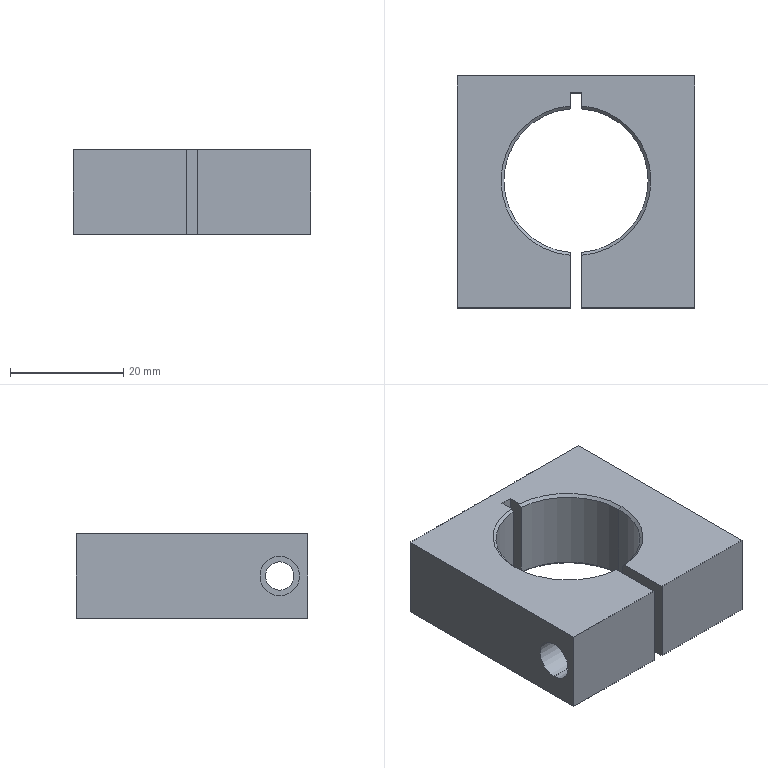Part | SolidWorks | features HoleWzd 3, Chamfer 2, ICE 2, Extrusion 1 | 1 solid | 33 faces | box 42 x 41 x 15 mm | volume 15925 mm3 | plane 12 | cylinder 11 | cone 10 | commonest cylinder face diameters 5 x6 25.5 x3 7 x2
STEP:
#1=CARTESIAN_POINT('',(8.25,22.5,0.5));
#2=VERTEX_POINT('',#1);
#3=CARTESIAN_POINT('',(20.,35.211,0.5));
#4=VERTEX_POINT('',#3);
#5=CARTESIAN_POINT('',(21.,22.5,0.5));
#6=DIRECTION('',(0.,0.,-1.));
#7=DIRECTION('',(-1.,0.,0.));
#8=AXIS2_PLACEMENT_3D('',#5,#6,#7);
#9=CIRCLE('',#8,12.75);
#10=EDGE_CURVE('',#2,#4,#9,.T.);
#11=ORIENTED_EDGE('',*,*,#10,.F.);
#12=CARTESIAN_POINT('',(7.75,22.5,0.));
#13=VERTEX_POINT('',#12);
#14=CARTESIAN_POINT('',(7.75,22.5,0.));
#15=DIRECTION('',(-0.7071,0.,-0.7071));
#16=VECTOR('',#15,1000.);
#17=LINE('',#14,#16);
#18=EDGE_CURVE('',#2,#13,#17,.T.);
#19=ORIENTED_EDGE('',*,*,#18,.T.);
#20=CARTESIAN_POINT('',(20.,35.712,0.));
#21=VERTEX_POINT('',#20);
#22=CARTESIAN_POINT('',(21.,22.5,0.));
#23=DIRECTION('',(0.,0.,1.));
#24=DIRECTION('',(-1.,0.,0.));
#25=AXIS2_PLACEMENT_3D('',#22,#23,#24);
#26=CIRCLE('',#25,13.25);
#27=EDGE_CURVE('',#21,#13,#26,.T.);
#28=ORIENTED_EDGE('',*,*,#27,.F.);
#29=CARTESIAN_POINT('',(20.,35.211,0.5));
#30=CARTESIAN_POINT('',(20.,35.378,0.3333));
#31=CARTESIAN_POINT('',(20.,35.545,0.1667));
#32=CARTESIAN_POINT('',(20.,35.712,0.));
#33=B_SPLINE_CURVE_WITH_KNOTS('',3,(#29,#30,#31,#32),.UNSPECIFIED.,.F.,.F.,(4,4),(0.,0.0007082),.UNSPECIFIED.);
#34=EDGE_CURVE('',#4,#21,#33,.T.);
#35=ORIENTED_EDGE('',*,*,#34,.F.);
#36=EDGE_LOOP('',(#11,#19,#28,#35));
#37=FACE_OUTER_BOUND('',#36,.T.);
#38=CARTESIAN_POINT('',(21.,22.5,0.));
#39=DIRECTION('',(0.,0.,-1.));
#40=DIRECTION('',(-1.,0.,0.));
#41=AXIS2_PLACEMENT_3D('',#38,#39,#40);
#42=CONICAL_SURFACE('',#41,13.25,0.7854);
#43=ADVANCED_FACE('',(#37),#42,.F.);
#44=CARTESIAN_POINT('',(33.75,22.5,14.5));
#45=VERTEX_POINT('',#44);
#46=CARTESIAN_POINT('',(22.,35.211,14.5));
#47=VERTEX_POINT('',#46);
#48=CARTESIAN_POINT('',(21.,22.5,14.5));
#49=DIRECTION('',(0.,0.,1.));
#50=DIRECTION('',(-1.,0.,0.));
#51=AXIS2_PLACEMENT_3D('',#48,#49,#50);
#52=CIRCLE('',#51,12.75);
#53=EDGE_CURVE('',#45,#47,#52,.T.);
#54=ORIENTED_EDGE('',*,*,#53,.F.);
#55=CARTESIAN_POINT('',(34.25,22.5,15.));
#56=VERTEX_POINT('',#55);
#57=CARTESIAN_POINT('',(33.75,22.5,14.5));
#58=DIRECTION('',(0.7071,0.,0.7071));
#59=VECTOR('',#58,1000.);
#60=LINE('',#57,#59);
#61=EDGE_CURVE('',#45,#56,#60,.T.);
#62=ORIENTED_EDGE('',*,*,#61,.T.);
#63=CARTESIAN_POINT('',(22.,35.712,15.));
#64=VERTEX_POINT('',#63);
#65=CARTESIAN_POINT('',(21.,22.5,15.));
#66=DIRECTION('',(0.,0.,-1.));
#67=DIRECTION('',(-1.,0.,0.));
#68=AXIS2_PLACEMENT_3D('',#65,#66,#67);
#69=CIRCLE('',#68,13.25);
#70=EDGE_CURVE('',#64,#56,#69,.T.);
#71=ORIENTED_EDGE('',*,*,#70,.F.);
#72=CARTESIAN_POINT('',(22.,35.211,14.5));
#73=CARTESIAN_POINT('',(22.,35.378,14.667));
#74=CARTESIAN_POINT('',(22.,35.545,14.833));
#75=CARTESIAN_POINT('',(22.,35.712,15.));
#76=B_SPLINE_CURVE_WITH_KNOTS('',3,(#72,#73,#74,#75),.UNSPECIFIED.,.F.,.F.,(4,4),(0.,0.0007082),.UNSPECIFIED.);
#77=EDGE_CURVE('',#47,#64,#76,.T.);
#78=ORIENTED_EDGE('',*,*,#77,.F.);
#79=EDGE_LOOP('',(#54,#62,#71,#78));
#80=FACE_OUTER_BOUND('',#79,.T.);
#81=CARTESIAN_POINT('',(21.,22.5,14.5));
#82=DIRECTION('',(0.,0.,1.));
#83=DIRECTION('',(1.,0.,0.));
#84=AXIS2_PLACEMENT_3D('',#81,#82,#83);
#85=CONICAL_SURFACE('',#84,12.75,0.7854);
#86=ADVANCED_FACE('',(#80),#85,.F.);
#87=CARTESIAN_POINT('',(42.,5.,5.));
#88=VERTEX_POINT('',#87);
#89=CARTESIAN_POINT('',(42.,5.,10.));
#90=VERTEX_POINT('',#89);
#91=CARTESIAN_POINT('',(42.,5.,7.5));
#92=DIRECTION('',(-1.,0.,0.));
#93=DIRECTION('',(0.,0.,1.));
#94=AXIS2_PLACEMENT_3D('',#91,#92,#93);
#95=CIRCLE('',#94,2.5);
#96=EDGE_CURVE('',#88,#90,#95,.T.);
#97=ORIENTED_EDGE('',*,*,#96,.F.);
#98=CARTESIAN_POINT('',(22.,5.,5.));
#99=VERTEX_POINT('',#98);
#100=CARTESIAN_POINT('',(22.,5.,5.));
#101=DIRECTION('',(-1.,0.,0.));
#102=VECTOR('',#101,1000.);
#103=LINE('',#100,#102);
#104=EDGE_CURVE('',#88,#99,#103,.T.);
#105=ORIENTED_EDGE('',*,*,#104,.T.);
#106=CARTESIAN_POINT('',(22.,5.,10.));
#107=VERTEX_POINT('',#106);
#108=CARTESIAN_POINT('',(22.,5.,7.5));
#109=DIRECTION('',(-1.,0.,0.));
#110=DIRECTION('',(0.,0.,1.));
#111=AXIS2_PLACEMENT_3D('',#108,#109,#110);
#112=CIRCLE('',#111,2.5);
#113=EDGE_CURVE('',#99,#107,#112,.T.);
#114=ORIENTED_EDGE('',*,*,#113,.T.);
#115=CARTESIAN_POINT('',(22.,5.,10.));
#116=DIRECTION('',(-1.,0.,0.));
#117=VECTOR('',#116,1000.);
#118=LINE('',#115,#117);
#119=EDGE_CURVE('',#90,#107,#118,.T.);
#120=ORIENTED_EDGE('',*,*,#119,.F.);
#121=EDGE_LOOP('',(#97,#105,#114,#120));
#122=FACE_OUTER_BOUND('',#121,.T.);
#123=CARTESIAN_POINT('',(22.,5.,7.5));
#124=DIRECTION('',(-1.,0.,0.));
#125=DIRECTION('',(0.,0.,1.));
#126=AXIS2_PLACEMENT_3D('',#123,#124,#125);
#127=CYLINDRICAL_SURFACE('',#126,2.5);
#128=ADVANCED_FACE('',(#122),#127,.F.);
#129=CARTESIAN_POINT('',(20.,5.,4.));
#130=VERTEX_POINT('',#129);
#131=CARTESIAN_POINT('',(20.,5.,11.));
#132=VERTEX_POINT('',#131);
#133=CARTESIAN_POINT('',(20.,5.,7.5));
#134=DIRECTION('',(-1.,0.,0.));
#135=DIRECTION('',(0.,-1.,0.));
#136=AXIS2_PLACEMENT_3D('',#133,#134,#135);
#137=CIRCLE('',#136,3.5);
#138=EDGE_CURVE('',#130,#132,#137,.T.);
#139=ORIENTED_EDGE('',*,*,#138,.F.);
#140=CARTESIAN_POINT('',(0.,5.,4.));
#141=VERTEX_POINT('',#140);
#142=CARTESIAN_POINT('',(0.,5.,4.));
#143=DIRECTION('',(-1.,0.,0.));
#144=VECTOR('',#143,1000.);
#145=LINE('',#142,#144);
#146=EDGE_CURVE('',#130,#141,#145,.T.);
#147=ORIENTED_EDGE('',*,*,#146,.T.);
#148=CARTESIAN_POINT('',(0.,5.,11.));
#149=VERTEX_POINT('',#148);
#150=CARTESIAN_POINT('',(0.,5.,7.5));
#151=DIRECTION('',(-1.,0.,0.));
#152=DIRECTION('',(0.,0.,1.));
#153=AXIS2_PLACEMENT_3D('',#150,#151,#152);
#154=CIRCLE('',#153,3.5);
#155=EDGE_CURVE('',#141,#149,#154,.T.);
#156=ORIENTED_EDGE('',*,*,#155,.T.);
#157=CARTESIAN_POINT('',(0.,5.,11.));
#158=DIRECTION('',(-1.,0.,0.));
#159=VECTOR('',#158,1000.);
#160=LINE('',#157,#159);
#161=EDGE_CURVE('',#132,#149,#160,.T.);
#162=ORIENTED_EDGE('',*,*,#161,.F.);
#163=EDGE_LOOP('',(#139,#147,#156,#162));
#164=FACE_OUTER_BOUND('',#163,.T.);
#165=CARTESIAN_POINT('',(0.,5.,7.5));
#166=DIRECTION('',(-1.,0.,0.));
#167=DIRECTION('',(0.,0.,1.));
#168=AXIS2_PLACEMENT_3D('',#165,#166,#167);
#169=CYLINDRICAL_SURFACE('',#168,3.5);
#170=ADVANCED_FACE('',(#164),#169,.F.);
#171=CARTESIAN_POINT('',(5.,24.,5.));
#172=VERTEX_POINT('',#171);
#173=CARTESIAN_POINT('',(5.,24.,10.));
#174=VERTEX_POINT('',#173);
#175=CARTESIAN_POINT('',(5.,24.,7.5));
#176=DIRECTION('',(0.,1.,0.));
#177=DIRECTION('',(0.,0.,1.));
#178=AXIS2_PLACEMENT_3D('',#175,#176,#177);
#179=CIRCLE('',#178,2.5);
#180=EDGE_CURVE('',#172,#174,#179,.T.);
#181=ORIENTED_EDGE('',*,*,#180,.F.);
#182=CARTESIAN_POINT('',(5.,41.,5.));
#183=VERTEX_POINT('',#182);
#184=CARTESIAN_POINT('',(5.,41.,5.));
#185=DIRECTION('',(0.,1.,0.));
#186=VECTOR('',#185,1000.);
#187=LINE('',#184,#186);
#188=EDGE_CURVE('',#172,#183,#187,.T.);
#189=ORIENTED_EDGE('',*,*,#188,.T.);
#190=CARTESIAN_POINT('',(5.,41.,10.));
#191=VERTEX_POINT('',#190);
#192=CARTESIAN_POINT('',(5.,41.,7.5));
#193=DIRECTION('',(0.,1.,0.));
#194=DIRECTION('',(0.,0.,1.));
#195=AXIS2_PLACEMENT_3D('',#192,#193,#194);
#196=CIRCLE('',#195,2.5);
#197=EDGE_CURVE('',#183,#191,#196,.T.);
#198=ORIENTED_EDGE('',*,*,#197,.T.);
#199=CARTESIAN_POINT('',(5.,41.,10.));
#200=DIRECTION('',(0.,1.,0.));
#201=VECTOR('',#200,1000.);
#202=LINE('',#199,#201);
#203=EDGE_CURVE('',#174,#191,#202,.T.);
#204=ORIENTED_EDGE('',*,*,#203,.F.);
#205=EDGE_LOOP('',(#181,#189,#198,#204));
#206=FACE_OUTER_BOUND('',#205,.T.);
#207=CARTESIAN_POINT('',(5.,41.,7.5));
#208=DIRECTION('',(0.,1.,0.));
#209=DIRECTION('',(0.,0.,1.));
#210=AXIS2_PLACEMENT_3D('',#207,#208,#209);
#211=CYLINDRICAL_SURFACE('',#210,2.5);
#212=ADVANCED_FACE('',(#206),#211,.F.);
#213=CARTESIAN_POINT('',(5.,22.498,7.5));
#214=VERTEX_POINT('',#213);
#215=CARTESIAN_POINT('',(5.,24.,10.));
#216=DIRECTION('',(0.,0.515,0.8572));
#217=VECTOR('',#216,1000.);
#218=LINE('',#215,#217);
#219=EDGE_CURVE('',#214,#174,#218,.T.);
#220=ORIENTED_EDGE('',*,*,#219,.F.);
#221=CARTESIAN_POINT('',(5.,24.,5.));
#222=DIRECTION('',(0.,0.515,-0.8572));
#223=VECTOR('',#222,1000.);
#224=LINE('',#221,#223);
#225=EDGE_CURVE('',#214,#172,#224,.T.);
#226=ORIENTED_EDGE('',*,*,#225,.T.);
#227=ORIENTED_EDGE('',*,*,#180,.T.);
#228=EDGE_LOOP('',(#220,#226,#227));
#229=FACE_OUTER_BOUND('',#228,.T.);
#230=CARTESIAN_POINT('',(5.,24.,7.5));
#231=DIRECTION('',(0.,1.,0.));
#232=DIRECTION('',(0.,0.,1.));
#233=AXIS2_PLACEMENT_3D('',#230,#231,#232);
#234=CONICAL_SURFACE('',#233,2.5,1.03);
#235=ADVANCED_FACE('',(#229),#234,.F.);
#236=CARTESIAN_POINT('',(37.,24.,5.));
#237=VERTEX_POINT('',#236);
#238=CARTESIAN_POINT('',(37.,24.,10.));
#239=VERTEX_POINT('',#238);
#240=CARTESIAN_POINT('',(37.,24.,7.5));
#241=DIRECTION('',(0.,1.,0.));
#242=DIRECTION('',(0.,0.,1.));
#243=AXIS2_PLACEMENT_3D('',#240,#241,#242);
#244=CIRCLE('',#243,2.5);
#245=EDGE_CURVE('',#237,#239,#244,.T.);
#246=ORIENTED_EDGE('',*,*,#245,.F.);
#247=CARTESIAN_POINT('',(37.,41.,5.));
#248=VERTEX_POINT('',#247);
#249=CARTESIAN_POINT('',(37.,41.,5.));
#250=DIRECTION('',(0.,1.,0.));
#251=VECTOR('',#250,1000.);
#252=LINE('',#249,#251);
#253=EDGE_CURVE('',#237,#248,#252,.T.);
#254=ORIENTED_EDGE('',*,*,#253,.T.);
#255=CARTESIAN_POINT('',(37.,41.,10.));
#256=VERTEX_POINT('',#255);
#257=CARTESIAN_POINT('',(37.,41.,7.5));
#258=DIRECTION('',(0.,1.,0.));
#259=DIRECTION('',(0.,0.,1.));
#260=AXIS2_PLACEMENT_3D('',#257,#258,#259);
#261=CIRCLE('',#260,2.5);
#262=EDGE_CURVE('',#248,#256,#261,.T.);
#263=ORIENTED_EDGE('',*,*,#262,.T.);
#264=CARTESIAN_POINT('',(37.,41.,10.));
#265=DIRECTION('',(0.,1.,0.));
#266=VECTOR('',#265,1000.);
#267=LINE('',#264,#266);
#268=EDGE_CURVE('',#239,#256,#267,.T.);
#269=ORIENTED_EDGE('',*,*,#268,.F.);
#270=EDGE_LOOP('',(#246,#254,#263,#269));
#271=FACE_OUTER_BOUND('',#270,.T.);
#272=CARTESIAN_POINT('',(37.,41.,7.5));
#273=DIRECTION('',(0.,1.,0.));
#274=DIRECTION('',(0.,0.,1.));
#275=AXIS2_PLACEMENT_3D('',#272,#273,#274);
#276=CYLINDRICAL_SURFACE('',#275,2.5);
#277=ADVANCED_FACE('',(#271),#276,.F.);
#278=CARTESIAN_POINT('',(37.,22.498,7.5));
#279=VERTEX_POINT('',#278);
#280=CARTESIAN_POINT('',(37.,24.,10.));
#281=DIRECTION('',(0.,0.515,0.8572));
#282=VECTOR('',#281,1000.);
#283=LINE('',#280,#282);
#284=EDGE_CURVE('',#279,#239,#283,.T.);
#285=ORIENTED_EDGE('',*,*,#284,.F.);
#286=CARTESIAN_POINT('',(37.,24.,5.));
#287=DIRECTION('',(0.,0.515,-0.8572));
#288=VECTOR('',#287,1000.);
#289=LINE('',#286,#288);
#290=EDGE_CURVE('',#279,#237,#289,.T.);
#291=ORIENTED_EDGE('',*,*,#290,.T.);
#292=ORIENTED_EDGE('',*,*,#245,.T.);
#293=EDGE_LOOP('',(#285,#291,#292));
#294=FACE_OUTER_BOUND('',#293,.T.);
#295=CARTESIAN_POINT('',(37.,24.,7.5));
#296=DIRECTION('',(0.,1.,0.));
#297=DIRECTION('',(0.,0.,1.));
#298=AXIS2_PLACEMENT_3D('',#295,#296,#297);
#299=CONICAL_SURFACE('',#298,2.5,1.03);
#300=ADVANCED_FACE('',(#294),#299,.F.);
#301=CARTESIAN_POINT('',(22.,35.211,0.5));
#302=VERTEX_POINT('',#301);
#303=CARTESIAN_POINT('',(33.75,22.5,0.5));
#304=VERTEX_POINT('',#303);
#305=CARTESIAN_POINT('',(21.,22.5,0.5));
#306=DIRECTION('',(0.,0.,-1.));
#307=DIRECTION('',(-1.,0.,0.));
#308=AXIS2_PLACEMENT_3D('',#305,#306,#307);
#309=CIRCLE('',#308,12.75);
#310=EDGE_CURVE('',#302,#304,#309,.T.);
#311=ORIENTED_EDGE('',*,*,#310,.T.);
#312=CARTESIAN_POINT('',(33.75,22.5,0.));
#313=DIRECTION('',(0.,0.,1.));
#314=VECTOR('',#313,1000.);
#315=LINE('',#312,#314);
#316=EDGE_CURVE('',#304,#45,#315,.T.);
#317=ORIENTED_EDGE('',*,*,#316,.T.);
#318=ORIENTED_EDGE('',*,*,#53,.T.);
#319=CARTESIAN_POINT('',(22.,35.211,0.));
#320=DIRECTION('',(0.,0.,-1.));
#321=VECTOR('',#320,1000.);
#322=LINE('',#319,#321);
#323=EDGE_CURVE('',#47,#302,#322,.T.);
#324=ORIENTED_EDGE('',*,*,#323,.T.);
#325=EDGE_LOOP('',(#311,#317,#318,#324));
#326=FACE_OUTER_BOUND('',#325,.T.);
#327=CARTESIAN_POINT('',(21.,22.5,0.));
#328=DIRECTION('',(0.,0.,1.));
#329=DIRECTION('',(1.,0.,0.));
#330=AXIS2_PLACEMENT_3D('',#327,#328,#329);
#331=CYLINDRICAL_SURFACE('',#330,12.75);
#332=ADVANCED_FACE('',(#326),#331,.F.);
#333=CARTESIAN_POINT('',(0.,0.,0.));
#334=VERTEX_POINT('',#333);
#335=CARTESIAN_POINT('',(20.,0.,0.));
#336=VERTEX_POINT('',#335);
#337=CARTESIAN_POINT('',(0.,0.,0.));
#338=DIRECTION('',(1.,0.,0.));
#339=VECTOR('',#338,1000.);
#340=LINE('',#337,#339);
#341=EDGE_CURVE('',#334,#336,#340,.T.);
#342=ORIENTED_EDGE('',*,*,#341,.T.);
#343=CARTESIAN_POINT('',(20.,0.,15.));
#344=VERTEX_POINT('',#343);
#345=CARTESIAN_POINT('',(20.,0.,0.));
#346=DIRECTION('',(0.,0.,1.));
#347=VECTOR('',#346,1000.);
#348=LINE('',#345,#347);
#349=EDGE_CURVE('',#336,#344,#348,.T.);
#350=ORIENTED_EDGE('',*,*,#349,.T.);
#351=CARTESIAN_POINT('',(0.,0.,15.));
#352=VERTEX_POINT('',#351);
#353=CARTESIAN_POINT('',(0.,0.,15.));
#354=DIRECTION('',(1.,0.,0.));
#355=VECTOR('',#354,1000.);
#356=LINE('',#353,#355);
#357=EDGE_CURVE('',#352,#344,#356,.T.);
#358=ORIENTED_EDGE('',*,*,#357,.F.);
#359=CARTESIAN_POINT('',(0.,0.,15.));
#360=DIRECTION('',(0.,0.,-1.));
#361=VECTOR('',#360,1000.);
#362=LINE('',#359,#361);
#363=EDGE_CURVE('',#352,#334,#362,.T.);
#364=ORIENTED_EDGE('',*,*,#363,.T.);
#365=EDGE_LOOP('',(#342,#350,#358,#364));
#366=FACE_OUTER_BOUND('',#365,.T.);
#367=CARTESIAN_POINT('',(0.,0.,15.));
#368=DIRECTION('',(0.,1.,0.));
#369=DIRECTION('',(0.,0.,1.));
#370=AXIS2_PLACEMENT_3D('',#367,#368,#369);
#371=PLANE('',#370);
#372=ADVANCED_FACE('',(#366),#371,.F.);
#373=CARTESIAN_POINT('',(20.,35.211,14.5));
#374=VERTEX_POINT('',#373);
#375=CARTESIAN_POINT('',(20.,35.211,0.));
#376=DIRECTION('',(0.,0.,1.));
#377=VECTOR('',#376,1000.);
#378=LINE('',#375,#377);
#379=EDGE_CURVE('',#4,#374,#378,.T.);
#380=ORIENTED_EDGE('',*,*,#379,.T.);
#381=CARTESIAN_POINT('',(20.,9.789,14.5));
#382=VERTEX_POINT('',#381);
#383=CARTESIAN_POINT('',(21.,22.5,14.5));
#384=DIRECTION('',(0.,0.,1.));
#385=DIRECTION('',(-1.,0.,0.));
#386=AXIS2_PLACEMENT_3D('',#383,#384,#385);
#387=CIRCLE('',#386,12.75);
#388=EDGE_CURVE('',#374,#382,#387,.T.);
#389=ORIENTED_EDGE('',*,*,#388,.T.);
#390=CARTESIAN_POINT('',(20.,9.789,0.5));
#391=VERTEX_POINT('',#390);
#392=CARTESIAN_POINT('',(20.,9.789,0.));
#393=DIRECTION('',(0.,0.,-1.));
#394=VECTOR('',#393,1000.);
#395=LINE('',#392,#394);
#396=EDGE_CURVE('',#382,#391,#395,.T.);
#397=ORIENTED_EDGE('',*,*,#396,.T.);
#398=CARTESIAN_POINT('',(21.,22.5,0.5));
#399=DIRECTION('',(0.,0.,-1.));
#400=DIRECTION('',(-1.,0.,0.));
#401=AXIS2_PLACEMENT_3D('',#398,#399,#400);
#402=CIRCLE('',#401,12.75);
#403=EDGE_CURVE('',#391,#2,#402,.T.);
#404=ORIENTED_EDGE('',*,*,#403,.T.);
#405=ORIENTED_EDGE('',*,*,#10,.T.);
#406=EDGE_LOOP('',(#380,#389,#397,#404,#405));
#407=FACE_OUTER_BOUND('',#406,.T.);
#408=CARTESIAN_POINT('',(21.,22.5,0.));
#409=DIRECTION('',(0.,0.,1.));
#410=DIRECTION('',(1.,0.,0.));
#411=AXIS2_PLACEMENT_3D('',#408,#409,#410);
#412=CYLINDRICAL_SURFACE('',#411,12.75);
#413=ADVANCED_FACE('',(#407),#412,.F.);
#414=CARTESIAN_POINT('',(0.,5.,7.5));
#415=DIRECTION('',(-1.,0.,0.));
#416=DIRECTION('',(0.,0.,1.));
#417=AXIS2_PLACEMENT_3D('',#414,#415,#416);
#418=CIRCLE('',#417,3.5);
#419=EDGE_CURVE('',#149,#141,#418,.T.);
#420=ORIENTED_EDGE('',*,*,#419,.F.);
#421=ORIENTED_EDGE('',*,*,#155,.F.);
#422=EDGE_LOOP('',(#420,#421));
#423=FACE_BOUND('',#422,.T.);
#424=CARTESIAN_POINT('',(0.,41.,0.));
#425=VERTEX_POINT('',#424);
#426=CARTESIAN_POINT('',(0.,0.,0.));
#427=DIRECTION('',(0.,-1.,0.));
#428=VECTOR('',#427,1000.);
#429=LINE('',#426,#428);
#430=EDGE_CURVE('',#425,#334,#429,.T.);
#431=ORIENTED_EDGE('',*,*,#430,.T.);
#432=ORIENTED_EDGE('',*,*,#363,.F.);
#433=CARTESIAN_POINT('',(0.,41.,15.));
#434=VERTEX_POINT('',#433);
#435=CARTESIAN_POINT('',(0.,0.,15.));
#436=DIRECTION('',(0.,-1.,0.));
#437=VECTOR('',#436,1000.);
#438=LINE('',#435,#437);
#439=EDGE_CURVE('',#434,#352,#438,.T.);
#440=ORIENTED_EDGE('',*,*,#439,.F.);
#441=CARTESIAN_POINT('',(0.,41.,15.));
#442=DIRECTION('',(0.,0.,-1.));
#443=VECTOR('',#442,1000.);
#444=LINE('',#441,#443);
#445=EDGE_CURVE('',#434,#425,#444,.T.);
#446=ORIENTED_EDGE('',*,*,#445,.T.);
#447=EDGE_LOOP('',(#431,#432,#440,#446));
#448=FACE_OUTER_BOUND('',#447,.T.);
#449=CARTESIAN_POINT('',(0.,0.,15.));
#450=DIRECTION('',(1.,0.,0.));
#451=DIRECTION('',(0.,0.,-1.));
#452=AXIS2_PLACEMENT_3D('',#449,#450,#451);
#453=PLANE('',#452);
#454=ADVANCED_FACE('',(#423,#448),#453,.F.);
#455=CARTESIAN_POINT('',(22.,0.,15.));
#456=VERTEX_POINT('',#455);
#457=CARTESIAN_POINT('',(42.,0.,15.));
#458=VERTEX_POINT('',#457);
#459=CARTESIAN_POINT('',(0.,0.,15.));
#460=DIRECTION('',(1.,0.,0.));
#461=VECTOR('',#460,1000.);
#462=LINE('',#459,#461);
#463=EDGE_CURVE('',#456,#458,#462,.T.);
#464=ORIENTED_EDGE('',*,*,#463,.F.);
#465=CARTESIAN_POINT('',(22.,0.,0.));
#466=VERTEX_POINT('',#465);
#467=CARTESIAN_POINT('',(22.,0.,0.));
#468=DIRECTION('',(0.,0.,1.));
#469=VECTOR('',#468,1000.);
#470=LINE('',#467,#469);
#471=EDGE_CURVE('',#466,#456,#470,.T.);
#472=ORIENTED_EDGE('',*,*,#471,.F.);
#473=CARTESIAN_POINT('',(42.,0.,0.));
#474=VERTEX_POINT('',#473);
#475=CARTESIAN_POINT('',(0.,0.,0.));
#476=DIRECTION('',(1.,0.,0.));
#477=VECTOR('',#476,1000.);
#478=LINE('',#475,#477);
#479=EDGE_CURVE('',#466,#474,#478,.T.);
#480=ORIENTED_EDGE('',*,*,#479,.T.);
#481=CARTESIAN_POINT('',(42.,0.,15.));
#482=DIRECTION('',(0.,0.,-1.));
#483=VECTOR('',#482,1000.);
#484=LINE('',#481,#483);
#485=EDGE_CURVE('',#458,#474,#484,.T.);
#486=ORIENTED_EDGE('',*,*,#485,.F.);
#487=EDGE_LOOP('',(#464,#472,#480,#486));
#488=FACE_OUTER_BOUND('',#487,.T.);
#489=CARTESIAN_POINT('',(0.,0.,15.));
#490=DIRECTION('',(0.,1.,0.));
#491=DIRECTION('',(0.,0.,1.));
#492=AXIS2_PLACEMENT_3D('',#489,#490,#491);
#493=PLANE('',#492);
#494=ADVANCED_FACE('',(#488),#493,.F.);
#495=CARTESIAN_POINT('',(42.,5.,7.5));
#496=DIRECTION('',(-1.,0.,0.));
#497=DIRECTION('',(0.,0.,1.));
#498=AXIS2_PLACEMENT_3D('',#495,#496,#497);
#499=CIRCLE('',#498,2.5);
#500=EDGE_CURVE('',#90,#88,#499,.T.);
#501=ORIENTED_EDGE('',*,*,#500,.T.);
#502=ORIENTED_EDGE('',*,*,#96,.T.);
#503=EDGE_LOOP('',(#501,#502));
#504=FACE_BOUND('',#503,.T.);
#505=CARTESIAN_POINT('',(42.,41.,0.));
#506=VERTEX_POINT('',#505);
#507=CARTESIAN_POINT('',(42.,0.,0.));
#508=DIRECTION('',(0.,1.,0.));
#509=VECTOR('',#508,1000.);
#510=LINE('',#507,#509);
#511=EDGE_CURVE('',#474,#506,#510,.T.);
#512=ORIENTED_EDGE('',*,*,#511,.T.);
#513=CARTESIAN_POINT('',(42.,41.,15.));
#514=VERTEX_POINT('',#513);
#515=CARTESIAN_POINT('',(42.,41.,15.));
#516=DIRECTION('',(0.,0.,-1.));
#517=VECTOR('',#516,1000.);
#518=LINE('',#515,#517);
#519=EDGE_CURVE('',#514,#506,#518,.T.);
#520=ORIENTED_EDGE('',*,*,#519,.F.);
#521=CARTESIAN_POINT('',(42.,0.,15.));
#522=DIRECTION('',(0.,1.,0.));
#523=VECTOR('',#522,1000.);
#524=LINE('',#521,#523);
#525=EDGE_CURVE('',#458,#514,#524,.T.);
#526=ORIENTED_EDGE('',*,*,#525,.F.);
#527=ORIENTED_EDGE('',*,*,#485,.T.);
#528=EDGE_LOOP('',(#512,#520,#526,#527));
#529=FACE_OUTER_BOUND('',#528,.T.);
#530=CARTESIAN_POINT('',(42.,0.,15.));
#531=DIRECTION('',(-1.,0.,0.));
#532=DIRECTION('',(0.,0.,1.));
#533=AXIS2_PLACEMENT_3D('',#530,#531,#532);
#534=PLANE('',#533);
#535=ADVANCED_FACE('',(#504,#529),#534,.F.);
#536=CARTESIAN_POINT('',(5.,41.,7.5));
#537=DIRECTION('',(0.,1.,0.));
#538=DIRECTION('',(0.,0.,1.));
#539=AXIS2_PLACEMENT_3D('',#536,#537,#538);
#540=CIRCLE('',#539,2.5);
#541=EDGE_CURVE('',#191,#183,#540,.T.);
#542=ORIENTED_EDGE('',*,*,#541,.F.);
#543=ORIENTED_EDGE('',*,*,#197,.F.);
#544=EDGE_LOOP('',(#542,#543));
#545=FACE_BOUND('',#544,.T.);
#546=CARTESIAN_POINT('',(37.,41.,7.5));
#547=DIRECTION('',(0.,1.,0.));
#548=DIRECTION('',(0.,0.,1.));
#549=AXIS2_PLACEMENT_3D('',#546,#547,#548);
#550=CIRCLE('',#549,2.5);
#551=EDGE_CURVE('',#256,#248,#550,.T.);
#552=ORIENTED_EDGE('',*,*,#551,.F.);
#553=ORIENTED_EDGE('',*,*,#262,.F.);
#554=EDGE_LOOP('',(#552,#553));
#555=FACE_BOUND('',#554,.T.);
#556=CARTESIAN_POINT('',(0.,41.,0.));
#557=DIRECTION('',(-1.,0.,0.));
#558=VECTOR('',#557,1000.);
#559=LINE('',#556,#558);
#560=EDGE_CURVE('',#506,#425,#559,.T.);
#561=ORIENTED_EDGE('',*,*,#560,.T.);
#562=ORIENTED_EDGE('',*,*,#445,.F.);
#563=CARTESIAN_POINT('',(0.,41.,15.));
#564=DIRECTION('',(-1.,0.,0.));
#565=VECTOR('',#564,1000.);
#566=LINE('',#563,#565);
#567=EDGE_CURVE('',#514,#434,#566,.T.);
#568=ORIENTED_EDGE('',*,*,#567,.F.);
#569=ORIENTED_EDGE('',*,*,#519,.T.);
#570=EDGE_LOOP('',(#561,#562,#568,#569));
#571=FACE_OUTER_BOUND('',#570,.T.);
#572=CARTESIAN_POINT('',(0.,41.,15.));
#573=DIRECTION('',(0.,-1.,0.));
#574=DIRECTION('',(0.,0.,-1.));
#575=AXIS2_PLACEMENT_3D('',#572,#573,#574);
#576=PLANE('',#575);
#577=ADVANCED_FACE('',(#545,#555,#571),#576,.F.);
#578=CARTESIAN_POINT('',(20.,9.288,15.));
#579=VERTEX_POINT('',#578);
#580=CARTESIAN_POINT('',(20.,0.,15.));
#581=DIRECTION('',(0.,-1.,0.));
#582=VECTOR('',#581,1000.);
#583=LINE('',#580,#582);
#584=EDGE_CURVE('',#579,#344,#583,.T.);
#585=ORIENTED_EDGE('',*,*,#584,.F.);
#586=CARTESIAN_POINT('',(20.,35.712,15.));
#587=VERTEX_POINT('',#586);
#588=CARTESIAN_POINT('',(21.,22.5,15.));
#589=DIRECTION('',(0.,0.,-1.));
#590=DIRECTION('',(-1.,0.,0.));
#591=AXIS2_PLACEMENT_3D('',#588,#589,#590);
#592=CIRCLE('',#591,13.25);
#593=EDGE_CURVE('',#579,#587,#592,.T.);
#594=ORIENTED_EDGE('',*,*,#593,.T.);
#595=CARTESIAN_POINT('',(20.,38.,15.));
#596=VERTEX_POINT('',#595);
#597=CARTESIAN_POINT('',(20.,0.,15.));
#598=DIRECTION('',(0.,-1.,0.));
#599=VECTOR('',#598,1000.);
#600=LINE('',#597,#599);
#601=EDGE_CURVE('',#596,#587,#600,.T.);
#602=ORIENTED_EDGE('',*,*,#601,.F.);
#603=CARTESIAN_POINT('',(22.,38.,15.));
#604=VERTEX_POINT('',#603);
#605=CARTESIAN_POINT('',(20.,38.,15.));
#606=DIRECTION('',(-1.,0.,0.));
#607=VECTOR('',#606,1000.);
#608=LINE('',#605,#607);
#609=EDGE_CURVE('',#604,#596,#608,.T.);
#610=ORIENTED_EDGE('',*,*,#609,.F.);
#611=CARTESIAN_POINT('',(22.,0.,15.));
#612=DIRECTION('',(0.,1.,0.));
#613=VECTOR('',#612,1000.);
#614=LINE('',#611,#613);
#615=EDGE_CURVE('',#64,#604,#614,.T.);
#616=ORIENTED_EDGE('',*,*,#615,.F.);
#617=ORIENTED_EDGE('',*,*,#70,.T.);
#618=CARTESIAN_POINT('',(22.,9.288,15.));
#619=VERTEX_POINT('',#618);
#620=CARTESIAN_POINT('',(21.,22.5,15.));
#621=DIRECTION('',(0.,0.,-1.));
#622=DIRECTION('',(-1.,0.,0.));
#623=AXIS2_PLACEMENT_3D('',#620,#621,#622);
#624=CIRCLE('',#623,13.25);
#625=EDGE_CURVE('',#56,#619,#624,.T.);
#626=ORIENTED_EDGE('',*,*,#625,.T.);
#627=CARTESIAN_POINT('',(22.,0.,15.));
#628=DIRECTION('',(0.,1.,0.));
#629=VECTOR('',#628,1000.);
#630=LINE('',#627,#629);
#631=EDGE_CURVE('',#456,#619,#630,.T.);
#632=ORIENTED_EDGE('',*,*,#631,.F.);
#633=ORIENTED_EDGE('',*,*,#463,.T.);
#634=ORIENTED_EDGE('',*,*,#525,.T.);
#635=ORIENTED_EDGE('',*,*,#567,.T.);
#636=ORIENTED_EDGE('',*,*,#439,.T.);
#637=ORIENTED_EDGE('',*,*,#357,.T.);
#638=EDGE_LOOP('',(#585,#594,#602,#610,#616,#617,#626,#632,#633,#634,#635,#636,#637));
#639=FACE_OUTER_BOUND('',#638,.T.);
#640=CARTESIAN_POINT('',(0.,0.,15.));
#641=DIRECTION('',(0.,0.,-1.));
#642=DIRECTION('',(-1.,0.,0.));
#643=AXIS2_PLACEMENT_3D('',#640,#641,#642);
#644=PLANE('',#643);
#645=ADVANCED_FACE('',(#639),#644,.F.);
#646=CARTESIAN_POINT('',(20.,38.,0.));
#647=VERTEX_POINT('',#646);
#648=CARTESIAN_POINT('',(20.,0.,0.));
#649=DIRECTION('',(0.,-1.,0.));
#650=VECTOR('',#649,1000.);
#651=LINE('',#648,#650);
#652=EDGE_CURVE('',#647,#21,#651,.T.);
#653=ORIENTED_EDGE('',*,*,#652,.T.);
#654=ORIENTED_EDGE('',*,*,#27,.T.);
#655=CARTESIAN_POINT('',(20.,9.288,0.));
#656=VERTEX_POINT('',#655);
#657=CARTESIAN_POINT('',(21.,22.5,0.));
#658=DIRECTION('',(0.,0.,1.));
#659=DIRECTION('',(-1.,0.,0.));
#660=AXIS2_PLACEMENT_3D('',#657,#658,#659);
#661=CIRCLE('',#660,13.25);
#662=EDGE_CURVE('',#13,#656,#661,.T.);
#663=ORIENTED_EDGE('',*,*,#662,.T.);
#664=CARTESIAN_POINT('',(20.,0.,0.));
#665=DIRECTION('',(0.,-1.,0.));
#666=VECTOR('',#665,1000.);
#667=LINE('',#664,#666);
#668=EDGE_CURVE('',#656,#336,#667,.T.);
#669=ORIENTED_EDGE('',*,*,#668,.T.);
#670=ORIENTED_EDGE('',*,*,#341,.F.);
#671=ORIENTED_EDGE('',*,*,#430,.F.);
#672=ORIENTED_EDGE('',*,*,#560,.F.);
#673=ORIENTED_EDGE('',*,*,#511,.F.);
#674=ORIENTED_EDGE('',*,*,#479,.F.);
#675=CARTESIAN_POINT('',(22.,9.288,0.));
#676=VERTEX_POINT('',#675);
#677=CARTESIAN_POINT('',(22.,0.,0.));
#678=DIRECTION('',(0.,1.,0.));
#679=VECTOR('',#678,1000.);
#680=LINE('',#677,#679);
#681=EDGE_CURVE('',#466,#676,#680,.T.);
#682=ORIENTED_EDGE('',*,*,#681,.T.);
#683=CARTESIAN_POINT('',(22.,35.712,0.));
#684=VERTEX_POINT('',#683);
#685=CARTESIAN_POINT('',(21.,22.5,0.));
#686=DIRECTION('',(0.,0.,1.));
#687=DIRECTION('',(-1.,0.,0.));
#688=AXIS2_PLACEMENT_3D('',#685,#686,#687);
#689=CIRCLE('',#688,13.25);
#690=EDGE_CURVE('',#676,#684,#689,.T.);
#691=ORIENTED_EDGE('',*,*,#690,.T.);
#692=CARTESIAN_POINT('',(22.,38.,0.));
#693=VERTEX_POINT('',#692);
#694=CARTESIAN_POINT('',(22.,0.,0.));
#695=DIRECTION('',(0.,1.,0.));
#696=VECTOR('',#695,1000.);
#697=LINE('',#694,#696);
#698=EDGE_CURVE('',#684,#693,#697,.T.);
#699=ORIENTED_EDGE('',*,*,#698,.T.);
#700=CARTESIAN_POINT('',(20.,38.,0.));
#701=DIRECTION('',(-1.,0.,0.));
#702=VECTOR('',#701,1000.);
#703=LINE('',#700,#702);
#704=EDGE_CURVE('',#693,#647,#703,.T.);
#705=ORIENTED_EDGE('',*,*,#704,.T.);
#706=EDGE_LOOP('',(#653,#654,#663,#669,#670,#671,#672,#673,#674,#682,#691,#699,#705));
#707=FACE_OUTER_BOUND('',#706,.T.);
#708=CARTESIAN_POINT('',(0.,0.,0.));
#709=DIRECTION('',(0.,0.,-1.));
#710=DIRECTION('',(-1.,0.,0.));
#711=AXIS2_PLACEMENT_3D('',#708,#709,#710);
#712=PLANE('',#711);
#713=ADVANCED_FACE('',(#707),#712,.T.);
#714=ORIENTED_EDGE('',*,*,#316,.F.);
#715=CARTESIAN_POINT('',(22.,9.789,0.5));
#716=VERTEX_POINT('',#715);
#717=CARTESIAN_POINT('',(21.,22.5,0.5));
#718=DIRECTION('',(0.,0.,-1.));
#719=DIRECTION('',(-1.,0.,0.));
#720=AXIS2_PLACEMENT_3D('',#717,#718,#719);
#721=CIRCLE('',#720,12.75);
#722=EDGE_CURVE('',#304,#716,#721,.T.);
#723=ORIENTED_EDGE('',*,*,#722,.T.);
#724=CARTESIAN_POINT('',(22.,9.789,14.5));
#725=VERTEX_POINT('',#724);
#726=CARTESIAN_POINT('',(22.,9.789,0.));
#727=DIRECTION('',(0.,0.,1.));
#728=VECTOR('',#727,1000.);
#729=LINE('',#726,#728);
#730=EDGE_CURVE('',#716,#725,#729,.T.);
#731=ORIENTED_EDGE('',*,*,#730,.T.);
#732=CARTESIAN_POINT('',(21.,22.5,14.5));
#733=DIRECTION('',(0.,0.,1.));
#734=DIRECTION('',(-1.,0.,0.));
#735=AXIS2_PLACEMENT_3D('',#732,#733,#734);
#736=CIRCLE('',#735,12.75);
#737=EDGE_CURVE('',#725,#45,#736,.T.);
#738=ORIENTED_EDGE('',*,*,#737,.T.);
#739=EDGE_LOOP('',(#714,#723,#731,#738));
#740=FACE_OUTER_BOUND('',#739,.T.);
#741=CARTESIAN_POINT('',(21.,22.5,0.));
#742=DIRECTION('',(0.,0.,1.));
#743=DIRECTION('',(1.,0.,0.));
#744=AXIS2_PLACEMENT_3D('',#741,#742,#743);
#745=CYLINDRICAL_SURFACE('',#744,12.75);
#746=ADVANCED_FACE('',(#740),#745,.F.);
#747=CARTESIAN_POINT('',(22.,5.,7.5));
#748=DIRECTION('',(-1.,0.,0.));
#749=DIRECTION('',(0.,0.,1.));
#750=AXIS2_PLACEMENT_3D('',#747,#748,#749);
#751=CIRCLE('',#750,2.5);
#752=EDGE_CURVE('',#107,#99,#751,.T.);
#753=ORIENTED_EDGE('',*,*,#752,.F.);
#754=ORIENTED_EDGE('',*,*,#113,.F.);
#755=EDGE_LOOP('',(#753,#754));
#756=FACE_BOUND('',#755,.T.);
#757=ORIENTED_EDGE('',*,*,#730,.F.);
#758=CARTESIAN_POINT('',(22.,9.789,0.5));
#759=CARTESIAN_POINT('',(22.,9.622,0.3333));
#760=CARTESIAN_POINT('',(22.,9.455,0.1667));
#761=CARTESIAN_POINT('',(22.,9.288,0.));
#762=B_SPLINE_CURVE_WITH_KNOTS('',3,(#758,#759,#760,#761),.UNSPECIFIED.,.F.,.F.,(4,4),(0.,0.0007082),.UNSPECIFIED.);
#763=EDGE_CURVE('',#716,#676,#762,.T.);
#764=ORIENTED_EDGE('',*,*,#763,.T.);
#765=ORIENTED_EDGE('',*,*,#681,.F.);
#766=ORIENTED_EDGE('',*,*,#471,.T.);
#767=ORIENTED_EDGE('',*,*,#631,.T.);
#768=CARTESIAN_POINT('',(22.,9.288,15.));
#769=CARTESIAN_POINT('',(22.,9.455,14.833));
#770=CARTESIAN_POINT('',(22.,9.622,14.667));
#771=CARTESIAN_POINT('',(22.,9.789,14.5));
#772=B_SPLINE_CURVE_WITH_KNOTS('',3,(#768,#769,#770,#771),.UNSPECIFIED.,.F.,.F.,(4,4),(0.,0.0007082),.UNSPECIFIED.);
#773=EDGE_CURVE('',#619,#725,#772,.T.);
#774=ORIENTED_EDGE('',*,*,#773,.T.);
#775=EDGE_LOOP('',(#757,#764,#765,#766,#767,#774));
#776=FACE_OUTER_BOUND('',#775,.T.);
#777=CARTESIAN_POINT('',(22.,0.,0.));
#778=DIRECTION('',(1.,0.,0.));
#779=DIRECTION('',(0.,0.,-1.));
#780=AXIS2_PLACEMENT_3D('',#777,#778,#779);
#781=PLANE('',#780);
#782=ADVANCED_FACE('',(#756,#776),#781,.F.);
#783=ORIENTED_EDGE('',*,*,#601,.T.);
#784=CARTESIAN_POINT('',(20.,35.712,15.));
#785=CARTESIAN_POINT('',(20.,35.545,14.833));
#786=CARTESIAN_POINT('',(20.,35.378,14.667));
#787=CARTESIAN_POINT('',(20.,35.211,14.5));
#788=B_SPLINE_CURVE_WITH_KNOTS('',3,(#784,#785,#786,#787),.UNSPECIFIED.,.F.,.F.,(4,4),(0.,0.0007082),.UNSPECIFIED.);
#789=EDGE_CURVE('',#587,#374,#788,.T.);
#790=ORIENTED_EDGE('',*,*,#789,.T.);
#791=ORIENTED_EDGE('',*,*,#379,.F.);
#792=ORIENTED_EDGE('',*,*,#34,.T.);
#793=ORIENTED_EDGE('',*,*,#652,.F.);
#794=CARTESIAN_POINT('',(20.,38.,0.));
#795=DIRECTION('',(0.,0.,1.));
#796=VECTOR('',#795,1000.);
#797=LINE('',#794,#796);
#798=EDGE_CURVE('',#647,#596,#797,.T.);
#799=ORIENTED_EDGE('',*,*,#798,.T.);
#800=EDGE_LOOP('',(#783,#790,#791,#792,#793,#799));
#801=FACE_OUTER_BOUND('',#800,.T.);
#802=CARTESIAN_POINT('',(20.,0.,0.));
#803=DIRECTION('',(-1.,0.,0.));
#804=DIRECTION('',(0.,-1.,0.));
#805=AXIS2_PLACEMENT_3D('',#802,#803,#804);
#806=PLANE('',#805);
#807=ADVANCED_FACE('',(#801),#806,.F.);
#808=ORIENTED_EDGE('',*,*,#698,.F.);
#809=CARTESIAN_POINT('',(22.,35.712,0.));
#810=CARTESIAN_POINT('',(22.,35.545,0.1667));
#811=CARTESIAN_POINT('',(22.,35.378,0.3333));
#812=CARTESIAN_POINT('',(22.,35.211,0.5));
#813=B_SPLINE_CURVE_WITH_KNOTS('',3,(#809,#810,#811,#812),.UNSPECIFIED.,.F.,.F.,(4,4),(0.,0.0007082),.UNSPECIFIED.);
#814=EDGE_CURVE('',#684,#302,#813,.T.);
#815=ORIENTED_EDGE('',*,*,#814,.T.);
#816=ORIENTED_EDGE('',*,*,#323,.F.);
#817=ORIENTED_EDGE('',*,*,#77,.T.);
#818=ORIENTED_EDGE('',*,*,#615,.T.);
#819=CARTESIAN_POINT('',(22.,38.,0.));
#820=DIRECTION('',(0.,0.,1.));
#821=VECTOR('',#820,1000.);
#822=LINE('',#819,#821);
#823=EDGE_CURVE('',#693,#604,#822,.T.);
#824=ORIENTED_EDGE('',*,*,#823,.F.);
#825=EDGE_LOOP('',(#808,#815,#816,#817,#818,#824));
#826=FACE_OUTER_BOUND('',#825,.T.);
#827=CARTESIAN_POINT('',(22.,0.,0.));
#828=DIRECTION('',(1.,0.,0.));
#829=DIRECTION('',(0.,0.,-1.));
#830=AXIS2_PLACEMENT_3D('',#827,#828,#829);
#831=PLANE('',#830);
#832=ADVANCED_FACE('',(#826),#831,.F.);
#833=ORIENTED_EDGE('',*,*,#609,.T.);
#834=ORIENTED_EDGE('',*,*,#798,.F.);
#835=ORIENTED_EDGE('',*,*,#704,.F.);
#836=ORIENTED_EDGE('',*,*,#823,.T.);
#837=EDGE_LOOP('',(#833,#834,#835,#836));
#838=FACE_OUTER_BOUND('',#837,.T.);
#839=CARTESIAN_POINT('',(20.,38.,0.));
#840=DIRECTION('',(0.,1.,0.));
#841=DIRECTION('',(0.,0.,1.));
#842=AXIS2_PLACEMENT_3D('',#839,#840,#841);
#843=PLANE('',#842);
#844=ADVANCED_FACE('',(#838),#843,.F.);
#845=CARTESIAN_POINT('',(20.,5.,7.5));
#846=DIRECTION('',(-1.,0.,0.));
#847=DIRECTION('',(0.,-1.,0.));
#848=AXIS2_PLACEMENT_3D('',#845,#846,#847);
#849=CIRCLE('',#848,3.5);
#850=EDGE_CURVE('',#132,#130,#849,.T.);
#851=ORIENTED_EDGE('',*,*,#850,.T.);
#852=ORIENTED_EDGE('',*,*,#138,.T.);
#853=EDGE_LOOP('',(#851,#852));
#854=FACE_BOUND('',#853,.T.);
#855=ORIENTED_EDGE('',*,*,#396,.F.);
#856=CARTESIAN_POINT('',(20.,9.789,14.5));
#857=CARTESIAN_POINT('',(20.,9.622,14.667));
#858=CARTESIAN_POINT('',(20.,9.455,14.833));
#859=CARTESIAN_POINT('',(20.,9.288,15.));
#860=B_SPLINE_CURVE_WITH_KNOTS('',3,(#856,#857,#858,#859),.UNSPECIFIED.,.F.,.F.,(4,4),(0.,0.0007082),.UNSPECIFIED.);
#861=EDGE_CURVE('',#382,#579,#860,.T.);
#862=ORIENTED_EDGE('',*,*,#861,.T.);
#863=ORIENTED_EDGE('',*,*,#584,.T.);
#864=ORIENTED_EDGE('',*,*,#349,.F.);
#865=ORIENTED_EDGE('',*,*,#668,.F.);
#866=CARTESIAN_POINT('',(20.,9.288,0.));
#867=CARTESIAN_POINT('',(20.,9.455,0.1667));
#868=CARTESIAN_POINT('',(20.,9.622,0.3333));
#869=CARTESIAN_POINT('',(20.,9.789,0.5));
#870=B_SPLINE_CURVE_WITH_KNOTS('',3,(#866,#867,#868,#869),.UNSPECIFIED.,.F.,.F.,(4,4),(0.,0.0007082),.UNSPECIFIED.);
#871=EDGE_CURVE('',#656,#391,#870,.T.);
#872=ORIENTED_EDGE('',*,*,#871,.T.);
#873=EDGE_LOOP('',(#855,#862,#863,#864,#865,#872));
#874=FACE_OUTER_BOUND('',#873,.T.);
#875=CARTESIAN_POINT('',(20.,0.,0.));
#876=DIRECTION('',(-1.,0.,0.));
#877=DIRECTION('',(0.,-1.,0.));
#878=AXIS2_PLACEMENT_3D('',#875,#876,#877);
#879=PLANE('',#878);
#880=ADVANCED_FACE('',(#854,#874),#879,.F.);
#881=ORIENTED_EDGE('',*,*,#290,.F.);
#882=ORIENTED_EDGE('',*,*,#284,.T.);
#883=CARTESIAN_POINT('',(37.,24.,7.5));
#884=DIRECTION('',(0.,1.,0.));
#885=DIRECTION('',(0.,0.,1.));
#886=AXIS2_PLACEMENT_3D('',#883,#884,#885);
#887=CIRCLE('',#886,2.5);
#888=EDGE_CURVE('',#239,#237,#887,.T.);
#889=ORIENTED_EDGE('',*,*,#888,.T.);
#890=EDGE_LOOP('',(#881,#882,#889));
#891=FACE_OUTER_BOUND('',#890,.T.);
#892=CARTESIAN_POINT('',(37.,24.,7.5));
#893=DIRECTION('',(0.,1.,0.));
#894=DIRECTION('',(0.,0.,1.));
#895=AXIS2_PLACEMENT_3D('',#892,#893,#894);
#896=CONICAL_SURFACE('',#895,2.5,1.03);
#897=ADVANCED_FACE('',(#891),#896,.F.);
#898=ORIENTED_EDGE('',*,*,#253,.F.);
#899=ORIENTED_EDGE('',*,*,#888,.F.);
#900=ORIENTED_EDGE('',*,*,#268,.T.);
#901=ORIENTED_EDGE('',*,*,#551,.T.);
#902=EDGE_LOOP('',(#898,#899,#900,#901));
#903=FACE_OUTER_BOUND('',#902,.T.);
#904=CARTESIAN_POINT('',(37.,41.,7.5));
#905=DIRECTION('',(0.,1.,0.));
#906=DIRECTION('',(0.,0.,1.));
#907=AXIS2_PLACEMENT_3D('',#904,#905,#906);
#908=CYLINDRICAL_SURFACE('',#907,2.5);
#909=ADVANCED_FACE('',(#903),#908,.F.);
#910=ORIENTED_EDGE('',*,*,#225,.F.);
#911=ORIENTED_EDGE('',*,*,#219,.T.);
#912=CARTESIAN_POINT('',(5.,24.,7.5));
#913=DIRECTION('',(0.,1.,0.));
#914=DIRECTION('',(0.,0.,1.));
#915=AXIS2_PLACEMENT_3D('',#912,#913,#914);
#916=CIRCLE('',#915,2.5);
#917=EDGE_CURVE('',#174,#172,#916,.T.);
#918=ORIENTED_EDGE('',*,*,#917,.T.);
#919=EDGE_LOOP('',(#910,#911,#918));
#920=FACE_OUTER_BOUND('',#919,.T.);
#921=CARTESIAN_POINT('',(5.,24.,7.5));
#922=DIRECTION('',(0.,1.,0.));
#923=DIRECTION('',(0.,0.,1.));
#924=AXIS2_PLACEMENT_3D('',#921,#922,#923);
#925=CONICAL_SURFACE('',#924,2.5,1.03);
#926=ADVANCED_FACE('',(#920),#925,.F.);
#927=ORIENTED_EDGE('',*,*,#188,.F.);
#928=ORIENTED_EDGE('',*,*,#917,.F.);
#929=ORIENTED_EDGE('',*,*,#203,.T.);
#930=ORIENTED_EDGE('',*,*,#541,.T.);
#931=EDGE_LOOP('',(#927,#928,#929,#930));
#932=FACE_OUTER_BOUND('',#931,.T.);
#933=CARTESIAN_POINT('',(5.,41.,7.5));
#934=DIRECTION('',(0.,1.,0.));
#935=DIRECTION('',(0.,0.,1.));
#936=AXIS2_PLACEMENT_3D('',#933,#934,#935);
#937=CYLINDRICAL_SURFACE('',#936,2.5);
#938=ADVANCED_FACE('',(#932),#937,.F.);
#939=ORIENTED_EDGE('',*,*,#146,.F.);
#940=ORIENTED_EDGE('',*,*,#850,.F.);
#941=ORIENTED_EDGE('',*,*,#161,.T.);
#942=ORIENTED_EDGE('',*,*,#419,.T.);
#943=EDGE_LOOP('',(#939,#940,#941,#942));
#944=FACE_OUTER_BOUND('',#943,.T.);
#945=CARTESIAN_POINT('',(0.,5.,7.5));
#946=DIRECTION('',(-1.,0.,0.));
#947=DIRECTION('',(0.,0.,1.));
#948=AXIS2_PLACEMENT_3D('',#945,#946,#947);
#949=CYLINDRICAL_SURFACE('',#948,3.5);
#950=ADVANCED_FACE('',(#944),#949,.F.);
#951=ORIENTED_EDGE('',*,*,#104,.F.);
#952=ORIENTED_EDGE('',*,*,#500,.F.);
#953=ORIENTED_EDGE('',*,*,#119,.T.);
#954=ORIENTED_EDGE('',*,*,#752,.T.);
#955=EDGE_LOOP('',(#951,#952,#953,#954));
#956=FACE_OUTER_BOUND('',#955,.T.);
#957=CARTESIAN_POINT('',(22.,5.,7.5));
#958=DIRECTION('',(-1.,0.,0.));
#959=DIRECTION('',(0.,0.,1.));
#960=AXIS2_PLACEMENT_3D('',#957,#958,#959);
#961=CYLINDRICAL_SURFACE('',#960,2.5);
#962=ADVANCED_FACE('',(#956),#961,.F.);
#963=ORIENTED_EDGE('',*,*,#763,.F.);
#964=ORIENTED_EDGE('',*,*,#722,.F.);
#965=ORIENTED_EDGE('',*,*,#310,.F.);
#966=ORIENTED_EDGE('',*,*,#814,.F.);
#967=ORIENTED_EDGE('',*,*,#690,.F.);
#968=EDGE_LOOP('',(#963,#964,#965,#966,#967));
#969=FACE_OUTER_BOUND('',#968,.T.);
#970=CARTESIAN_POINT('',(21.,22.5,0.));
#971=DIRECTION('',(0.,0.,-1.));
#972=DIRECTION('',(-1.,0.,0.));
#973=AXIS2_PLACEMENT_3D('',#970,#971,#972);
#974=CONICAL_SURFACE('',#973,13.25,0.7854);
#975=ADVANCED_FACE('',(#969),#974,.F.);
#976=ORIENTED_EDGE('',*,*,#61,.F.);
#977=ORIENTED_EDGE('',*,*,#737,.F.);
#978=ORIENTED_EDGE('',*,*,#773,.F.);
#979=ORIENTED_EDGE('',*,*,#625,.F.);
#980=EDGE_LOOP('',(#976,#977,#978,#979));
#981=FACE_OUTER_BOUND('',#980,.T.);
#982=CARTESIAN_POINT('',(21.,22.5,14.5));
#983=DIRECTION('',(0.,0.,1.));
#984=DIRECTION('',(1.,0.,0.));
#985=AXIS2_PLACEMENT_3D('',#982,#983,#984);
#986=CONICAL_SURFACE('',#985,12.75,0.7854);
#987=ADVANCED_FACE('',(#981),#986,.F.);
#988=ORIENTED_EDGE('',*,*,#789,.F.);
#989=ORIENTED_EDGE('',*,*,#593,.F.);
#990=ORIENTED_EDGE('',*,*,#861,.F.);
#991=ORIENTED_EDGE('',*,*,#388,.F.);
#992=EDGE_LOOP('',(#988,#989,#990,#991));
#993=FACE_OUTER_BOUND('',#992,.T.);
#994=CARTESIAN_POINT('',(21.,22.5,14.5));
#995=DIRECTION('',(0.,0.,1.));
#996=DIRECTION('',(1.,0.,0.));
#997=AXIS2_PLACEMENT_3D('',#994,#995,#996);
#998=CONICAL_SURFACE('',#997,12.75,0.7854);
#999=ADVANCED_FACE('',(#993),#998,.F.);
#1000=ORIENTED_EDGE('',*,*,#18,.F.);
#1001=ORIENTED_EDGE('',*,*,#403,.F.);
#1002=ORIENTED_EDGE('',*,*,#871,.F.);
#1003=ORIENTED_EDGE('',*,*,#662,.F.);
#1004=EDGE_LOOP('',(#1000,#1001,#1002,#1003));
#1005=FACE_OUTER_BOUND('',#1004,.T.);
#1006=CARTESIAN_POINT('',(21.,22.5,0.));
#1007=DIRECTION('',(0.,0.,-1.));
#1008=DIRECTION('',(-1.,0.,0.));
#1009=AXIS2_PLACEMENT_3D('',#1006,#1007,#1008);
#1010=CONICAL_SURFACE('',#1009,13.25,0.7854);
#1011=ADVANCED_FACE('',(#1005),#1010,.F.);
#1012=CLOSED_SHELL('',(#43,#86,#128,#170,#212,#235,#277,#300,#332,#372,#413,#454,#494,#535,#577,#645,#713,#746,#782,#807,#832,#844,#880,#897,#909,#926,#938,#950,#962,#975,#987,#999,#1011));
#1013=MANIFOLD_SOLID_BREP('',#1012);
#1014=CARTESIAN_POINT('',(0.,0.,0.));
#1015=DIRECTION('',(0.,0.,1.));
#1016=DIRECTION('',(1.,0.,0.));
#1017=AXIS2_PLACEMENT_3D('',#1014,#1015,#1016);
#1018=(LENGTH_UNIT()NAMED_UNIT(*)SI_UNIT(.MILLI.,.METRE.));
#1019=UNCERTAINTY_MEASURE_WITH_UNIT(LENGTH_MEASURE(0.00001),#1018,'','');
#1020=(NAMED_UNIT(*)PLANE_ANGLE_UNIT()SI_UNIT($,.RADIAN.));
#1021=(NAMED_UNIT(*)SI_UNIT($,.STERADIAN.)SOLID_ANGLE_UNIT());
#1022=(GEOMETRIC_REPRESENTATION_CONTEXT(3)GLOBAL_UNCERTAINTY_ASSIGNED_CONTEXT((#1019))GLOBAL_UNIT_ASSIGNED_CONTEXT((#1018,#1020,#1021))REPRESENTATION_CONTEXT('',''));
#1023=ADVANCED_BREP_SHAPE_REPRESENTATION('',(#1013,#1017),#1022);